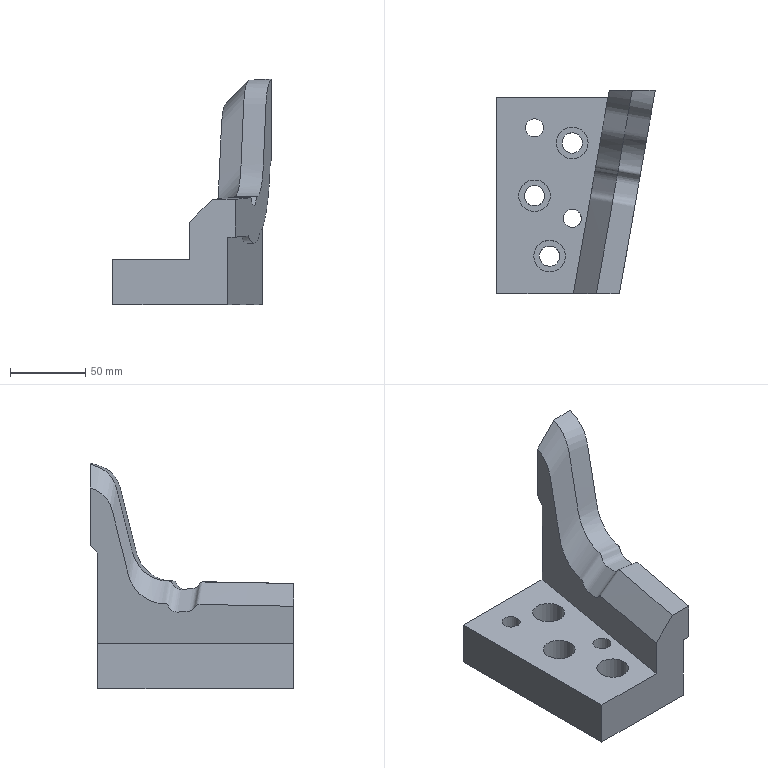Part | NX | features solid 2 | 1 solid | 24 faces | box 105.001 x 134.807 x 149.46 mm | volume 494026 mm3 | spline 8 | plane 8 | cylinder 8 | commonest cylinder face diameters 13.5 x3 21 x3 12 x2